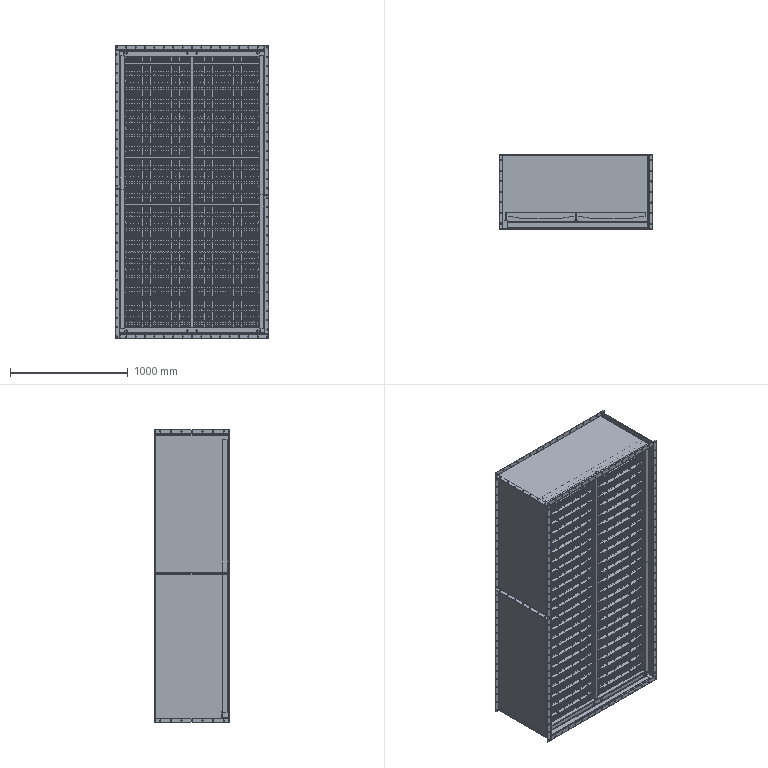Part | SolidWorks | features ReferencePattern 7, LocalLPattern 1 | 411 solids | 18942 faces | volume 57196333 mm3 | plane 12212 | cylinder 4846 | cone 1728 | torus 144 | spline 12 | commonest cylinder face diameters 10 x3216 8 x288 8.1 x216 12.277 x216 11 x146 9 x144